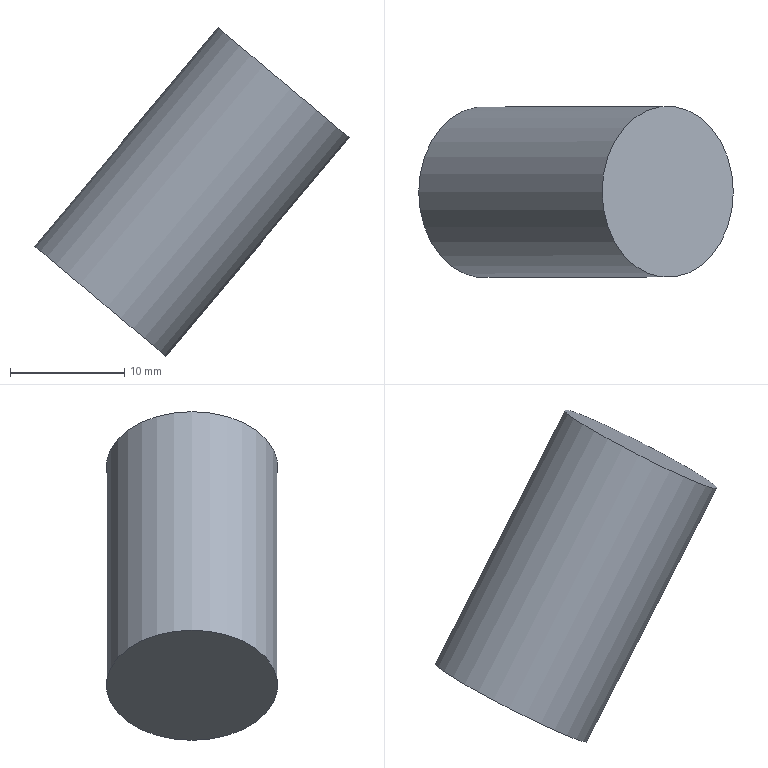Part | NX | features solid 2 | 1 solid | 3 faces | box 27.56 x 15 x 28.793 mm | volume 4418 mm3 | plane 2 | cylinder 1 | commonest cylinder face diameters 15 x1
STEP:
#1=CARTESIAN_POINT('',(905.851,500.,-98.91));
#2=VERTEX_POINT('',#1);
#3=CARTESIAN_POINT('',(900.105,500.,-94.089));
#4=DIRECTION('',(-0.6428,0.,-0.766));
#5=DIRECTION('',(0.766,0.,-0.6428));
#6=AXIS2_PLACEMENT_3D('',#3,#4,#5);
#7=CIRCLE('',#6,7.5);
#8=EDGE_CURVE('',#2,#2,#7,.T.);
#9=ORIENTED_EDGE('',*,*,#8,.F.);
#10=EDGE_LOOP('',(#9));
#11=FACE_BOUND('',#10,.T.);
#12=CARTESIAN_POINT('',(900.105,500.,-94.089));
#13=DIRECTION('',(0.6428,0.,0.766));
#14=DIRECTION('',(0.,-1.,0.));
#15=AXIS2_PLACEMENT_3D('',#12,#13,#14);
#16=PLANE('',#15);
#17=ADVANCED_FACE('',(#11),#16,.T.);
#18=CARTESIAN_POINT('',(889.781,500.,-118.061));
#19=VERTEX_POINT('',#18);
#20=CARTESIAN_POINT('',(884.036,500.,-113.24));
#21=DIRECTION('',(-0.6428,0.,-0.766));
#22=DIRECTION('',(0.766,0.,-0.6428));
#23=AXIS2_PLACEMENT_3D('',#20,#21,#22);
#24=CIRCLE('',#23,7.5);
#25=EDGE_CURVE('',#19,#19,#24,.T.);
#26=ORIENTED_EDGE('',*,*,#25,.F.);
#27=EDGE_LOOP('',(#26));
#28=FACE_BOUND('',#27,.T.);
#29=ORIENTED_EDGE('',*,*,#8,.T.);
#30=EDGE_LOOP('',(#29));
#31=FACE_BOUND('',#30,.T.);
#32=CARTESIAN_POINT('',(896.249,500.,-98.685));
#33=DIRECTION('',(-0.6428,0.,-0.766));
#34=DIRECTION('',(0.,1.,0.));
#35=AXIS2_PLACEMENT_3D('',#32,#33,#34);
#36=CYLINDRICAL_SURFACE('',#35,7.5);
#37=ADVANCED_FACE('',(#28,#31),#36,.T.);
#38=ORIENTED_EDGE('',*,*,#25,.T.);
#39=EDGE_LOOP('',(#38));
#40=FACE_BOUND('',#39,.T.);
#41=CARTESIAN_POINT('',(884.036,500.,-113.24));
#42=DIRECTION('',(0.6428,0.,0.766));
#43=DIRECTION('',(0.,-1.,0.));
#44=AXIS2_PLACEMENT_3D('',#41,#42,#43);
#45=PLANE('',#44);
#46=ADVANCED_FACE('',(#40),#45,.F.);
#47=CLOSED_SHELL('',(#17,#37,#46));
#48=MANIFOLD_SOLID_BREP('',#47);
#49=(LENGTH_UNIT()NAMED_UNIT(*)SI_UNIT(.MILLI.,.METRE.));
#50=UNCERTAINTY_MEASURE_WITH_UNIT(LENGTH_MEASURE(0.00001),#49,'','');
#51=(NAMED_UNIT(*)PLANE_ANGLE_UNIT()SI_UNIT($,.RADIAN.));
#52=(NAMED_UNIT(*)SI_UNIT($,.STERADIAN.)SOLID_ANGLE_UNIT());
#53=(GEOMETRIC_REPRESENTATION_CONTEXT(3)GLOBAL_UNCERTAINTY_ASSIGNED_CONTEXT((#50))GLOBAL_UNIT_ASSIGNED_CONTEXT((#49,#51,#52))REPRESENTATION_CONTEXT('',''));
#54=ADVANCED_BREP_SHAPE_REPRESENTATION('',(#48),#53);